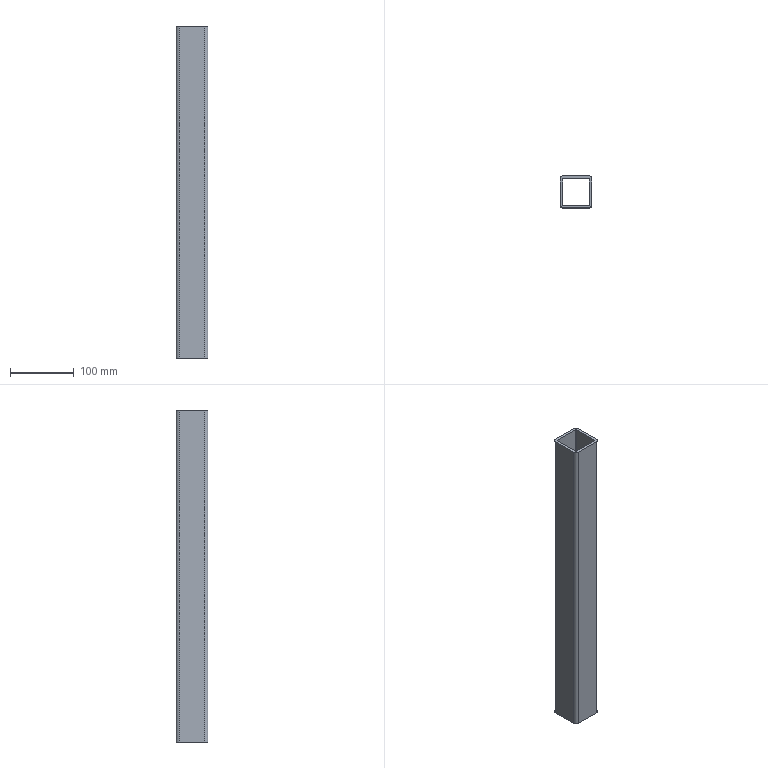Part | STEP file | Square steel 50×50×132 | 1 solid | 22 faces | box 50 x 50 x 520 mm | volume 371896 mm3 | cylinder 12 | plane 10 | commonest cylinder face diameters 2 x4 4.2 x4 10 x4